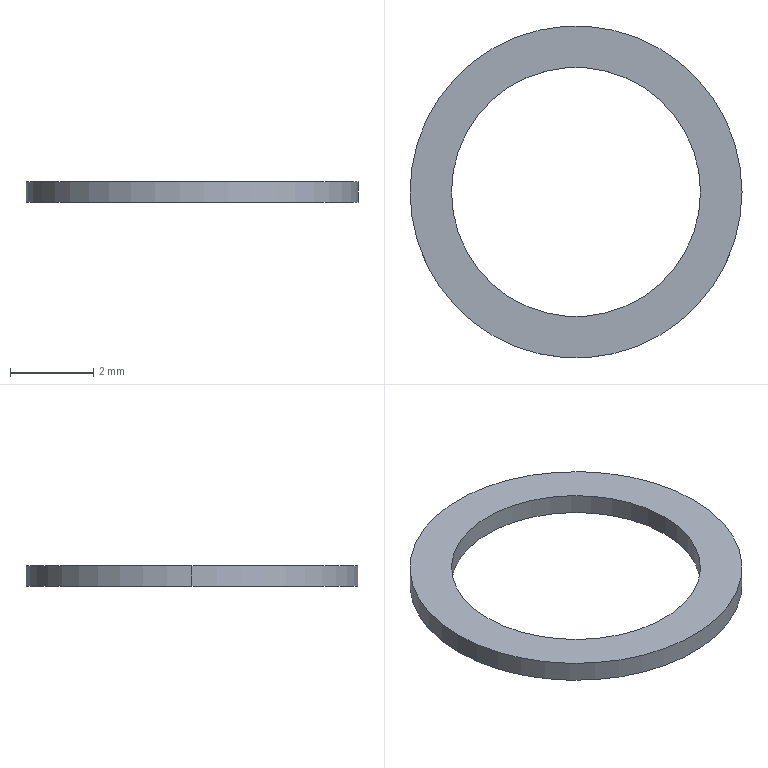Part | SolidWorks | features Extrusion 1 | 1 solid | 6 faces | box 8 x 8 x 0.5 mm | volume 10.996 mm3 | cylinder 4 | plane 2 | commonest cylinder face diameters 6 x2 8 x2
STEP:
#1=CARTESIAN_POINT('',(-3.,0.,0.5));
#2=VERTEX_POINT('',#1);
#3=CARTESIAN_POINT('',(3.,0.,0.5));
#4=VERTEX_POINT('',#3);
#5=CARTESIAN_POINT('',(0.,0.,0.5));
#6=DIRECTION('',(0.,0.,1.));
#7=DIRECTION('',(1.,0.,0.));
#8=AXIS2_PLACEMENT_3D('',#5,#6,#7);
#9=CIRCLE('',#8,3.);
#10=EDGE_CURVE('',#2,#4,#9,.T.);
#11=ORIENTED_EDGE('',*,*,#10,.T.);
#12=CARTESIAN_POINT('',(3.,0.,0.));
#13=VERTEX_POINT('',#12);
#14=CARTESIAN_POINT('',(3.,0.,0.5));
#15=DIRECTION('',(0.,0.,-1.));
#16=VECTOR('',#15,1000.);
#17=LINE('',#14,#16);
#18=EDGE_CURVE('',#4,#13,#17,.T.);
#19=ORIENTED_EDGE('',*,*,#18,.T.);
#20=CARTESIAN_POINT('',(-3.,0.,0.));
#21=VERTEX_POINT('',#20);
#22=CARTESIAN_POINT('',(0.,0.,0.));
#23=DIRECTION('',(0.,0.,1.));
#24=DIRECTION('',(1.,0.,0.));
#25=AXIS2_PLACEMENT_3D('',#22,#23,#24);
#26=CIRCLE('',#25,3.);
#27=EDGE_CURVE('',#21,#13,#26,.T.);
#28=ORIENTED_EDGE('',*,*,#27,.F.);
#29=CARTESIAN_POINT('',(-3.,0.,0.5));
#30=DIRECTION('',(0.,0.,-1.));
#31=VECTOR('',#30,1000.);
#32=LINE('',#29,#31);
#33=EDGE_CURVE('',#2,#21,#32,.T.);
#34=ORIENTED_EDGE('',*,*,#33,.F.);
#35=EDGE_LOOP('',(#11,#19,#28,#34));
#36=FACE_OUTER_BOUND('',#35,.T.);
#37=CARTESIAN_POINT('',(0.,0.,0.5));
#38=DIRECTION('',(0.,0.,-1.));
#39=DIRECTION('',(-1.,0.,0.));
#40=AXIS2_PLACEMENT_3D('',#37,#38,#39);
#41=CYLINDRICAL_SURFACE('',#40,3.);
#42=ADVANCED_FACE('',(#36),#41,.F.);
#43=CARTESIAN_POINT('',(4.,0.,0.5));
#44=VERTEX_POINT('',#43);
#45=CARTESIAN_POINT('',(-4.,0.,0.5));
#46=VERTEX_POINT('',#45);
#47=CARTESIAN_POINT('',(0.,0.,0.5));
#48=DIRECTION('',(0.,0.,1.));
#49=DIRECTION('',(1.,0.,0.));
#50=AXIS2_PLACEMENT_3D('',#47,#48,#49);
#51=CIRCLE('',#50,4.);
#52=EDGE_CURVE('',#44,#46,#51,.T.);
#53=ORIENTED_EDGE('',*,*,#52,.F.);
#54=CARTESIAN_POINT('',(4.,0.,0.));
#55=VERTEX_POINT('',#54);
#56=CARTESIAN_POINT('',(4.,0.,0.5));
#57=DIRECTION('',(0.,0.,-1.));
#58=VECTOR('',#57,1000.);
#59=LINE('',#56,#58);
#60=EDGE_CURVE('',#44,#55,#59,.T.);
#61=ORIENTED_EDGE('',*,*,#60,.T.);
#62=CARTESIAN_POINT('',(-4.,0.,0.));
#63=VERTEX_POINT('',#62);
#64=CARTESIAN_POINT('',(0.,0.,0.));
#65=DIRECTION('',(0.,0.,1.));
#66=DIRECTION('',(1.,0.,0.));
#67=AXIS2_PLACEMENT_3D('',#64,#65,#66);
#68=CIRCLE('',#67,4.);
#69=EDGE_CURVE('',#55,#63,#68,.T.);
#70=ORIENTED_EDGE('',*,*,#69,.T.);
#71=CARTESIAN_POINT('',(-4.,0.,0.5));
#72=DIRECTION('',(0.,0.,-1.));
#73=VECTOR('',#72,1000.);
#74=LINE('',#71,#73);
#75=EDGE_CURVE('',#46,#63,#74,.T.);
#76=ORIENTED_EDGE('',*,*,#75,.F.);
#77=EDGE_LOOP('',(#53,#61,#70,#76));
#78=FACE_OUTER_BOUND('',#77,.T.);
#79=CARTESIAN_POINT('',(0.,0.,0.5));
#80=DIRECTION('',(0.,0.,-1.));
#81=DIRECTION('',(-1.,0.,0.));
#82=AXIS2_PLACEMENT_3D('',#79,#80,#81);
#83=CYLINDRICAL_SURFACE('',#82,4.);
#84=ADVANCED_FACE('',(#78),#83,.T.);
#85=CARTESIAN_POINT('',(0.,0.,0.5));
#86=DIRECTION('',(0.,0.,1.));
#87=DIRECTION('',(1.,0.,0.));
#88=AXIS2_PLACEMENT_3D('',#85,#86,#87);
#89=CIRCLE('',#88,4.);
#90=EDGE_CURVE('',#46,#44,#89,.T.);
#91=ORIENTED_EDGE('',*,*,#90,.T.);
#92=ORIENTED_EDGE('',*,*,#52,.T.);
#93=EDGE_LOOP('',(#91,#92));
#94=FACE_OUTER_BOUND('',#93,.T.);
#95=ORIENTED_EDGE('',*,*,#10,.F.);
#96=CARTESIAN_POINT('',(0.,0.,0.5));
#97=DIRECTION('',(0.,0.,1.));
#98=DIRECTION('',(1.,0.,0.));
#99=AXIS2_PLACEMENT_3D('',#96,#97,#98);
#100=CIRCLE('',#99,3.);
#101=EDGE_CURVE('',#4,#2,#100,.T.);
#102=ORIENTED_EDGE('',*,*,#101,.F.);
#103=EDGE_LOOP('',(#95,#102));
#104=FACE_BOUND('',#103,.T.);
#105=CARTESIAN_POINT('',(0.,0.,0.5));
#106=DIRECTION('',(0.,0.,1.));
#107=DIRECTION('',(1.,0.,0.));
#108=AXIS2_PLACEMENT_3D('',#105,#106,#107);
#109=PLANE('',#108);
#110=ADVANCED_FACE('',(#94,#104),#109,.T.);
#111=CARTESIAN_POINT('',(0.,0.,0.));
#112=DIRECTION('',(0.,0.,1.));
#113=DIRECTION('',(1.,0.,0.));
#114=AXIS2_PLACEMENT_3D('',#111,#112,#113);
#115=CIRCLE('',#114,4.);
#116=EDGE_CURVE('',#63,#55,#115,.T.);
#117=ORIENTED_EDGE('',*,*,#116,.F.);
#118=ORIENTED_EDGE('',*,*,#69,.F.);
#119=EDGE_LOOP('',(#117,#118));
#120=FACE_OUTER_BOUND('',#119,.T.);
#121=ORIENTED_EDGE('',*,*,#27,.T.);
#122=CARTESIAN_POINT('',(0.,0.,0.));
#123=DIRECTION('',(0.,0.,1.));
#124=DIRECTION('',(1.,0.,0.));
#125=AXIS2_PLACEMENT_3D('',#122,#123,#124);
#126=CIRCLE('',#125,3.);
#127=EDGE_CURVE('',#13,#21,#126,.T.);
#128=ORIENTED_EDGE('',*,*,#127,.T.);
#129=EDGE_LOOP('',(#121,#128));
#130=FACE_BOUND('',#129,.T.);
#131=CARTESIAN_POINT('',(0.,0.,0.));
#132=DIRECTION('',(0.,0.,1.));
#133=DIRECTION('',(1.,0.,0.));
#134=AXIS2_PLACEMENT_3D('',#131,#132,#133);
#135=PLANE('',#134);
#136=ADVANCED_FACE('',(#120,#130),#135,.F.);
#137=ORIENTED_EDGE('',*,*,#60,.F.);
#138=ORIENTED_EDGE('',*,*,#90,.F.);
#139=ORIENTED_EDGE('',*,*,#75,.T.);
#140=ORIENTED_EDGE('',*,*,#116,.T.);
#141=EDGE_LOOP('',(#137,#138,#139,#140));
#142=FACE_OUTER_BOUND('',#141,.T.);
#143=CARTESIAN_POINT('',(0.,0.,0.5));
#144=DIRECTION('',(0.,0.,-1.));
#145=DIRECTION('',(-1.,0.,0.));
#146=AXIS2_PLACEMENT_3D('',#143,#144,#145);
#147=CYLINDRICAL_SURFACE('',#146,4.);
#148=ADVANCED_FACE('',(#142),#147,.T.);
#149=ORIENTED_EDGE('',*,*,#18,.F.);
#150=ORIENTED_EDGE('',*,*,#101,.T.);
#151=ORIENTED_EDGE('',*,*,#33,.T.);
#152=ORIENTED_EDGE('',*,*,#127,.F.);
#153=EDGE_LOOP('',(#149,#150,#151,#152));
#154=FACE_OUTER_BOUND('',#153,.T.);
#155=CARTESIAN_POINT('',(0.,0.,0.5));
#156=DIRECTION('',(0.,0.,-1.));
#157=DIRECTION('',(-1.,0.,0.));
#158=AXIS2_PLACEMENT_3D('',#155,#156,#157);
#159=CYLINDRICAL_SURFACE('',#158,3.);
#160=ADVANCED_FACE('',(#154),#159,.F.);
#161=CLOSED_SHELL('',(#42,#84,#110,#136,#148,#160));
#162=MANIFOLD_SOLID_BREP('',#161);
#163=CARTESIAN_POINT('',(0.,0.,0.));
#164=DIRECTION('',(0.,0.,1.));
#165=DIRECTION('',(1.,0.,0.));
#166=AXIS2_PLACEMENT_3D('',#163,#164,#165);
#167=(LENGTH_UNIT()NAMED_UNIT(*)SI_UNIT(.MILLI.,.METRE.));
#168=UNCERTAINTY_MEASURE_WITH_UNIT(LENGTH_MEASURE(0.00001),#167,'','');
#169=(NAMED_UNIT(*)PLANE_ANGLE_UNIT()SI_UNIT($,.RADIAN.));
#170=(NAMED_UNIT(*)SI_UNIT($,.STERADIAN.)SOLID_ANGLE_UNIT());
#171=(GEOMETRIC_REPRESENTATION_CONTEXT(3)GLOBAL_UNCERTAINTY_ASSIGNED_CONTEXT((#168))GLOBAL_UNIT_ASSIGNED_CONTEXT((#167,#169,#170))REPRESENTATION_CONTEXT('',''));
#172=ADVANCED_BREP_SHAPE_REPRESENTATION('',(#162,#166),#171);